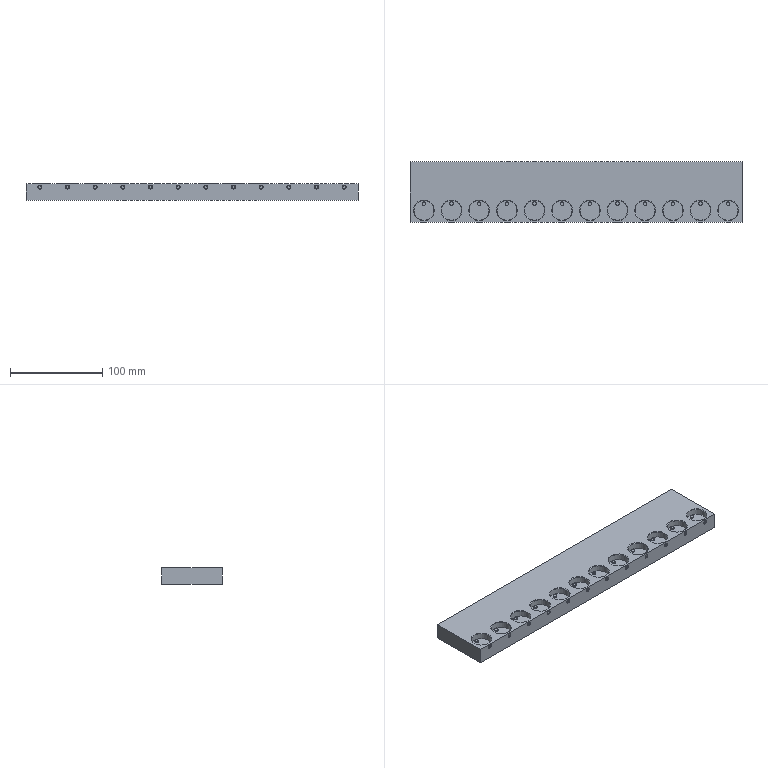NC program | NX | posted with a generic post | part box 360 x 66 x 17.6 mm
Lines 4604 to 5333 of 61781:
(2 , TOOL : D1-T2)
N9140 T02 M6
N9142 G54
N9144 G17 G0 G90 X-15.846 Y-13.281 B0. C0. S8000 M3
N9146 G43 Z100. H2
N9148 G94 G1 Z-5.5 F5000.
N9150 G3 X-15.846 Y-13.281 Z-5.515 I0.443 J0.081 F2000.
N9152 X-15.846 Y-13.281 Z-5.53 I0.443 J0.081
N9154 X-15.846 Y-13.281 Z-5.544 I0.443 J0.081
N9156 X-15.846 Y-13.281 Z-5.559 I0.443 J0.081
N9158 X-15.846 Y-13.281 Z-5.574 I0.443 J0.081
N9160 X-15.846 Y-13.281 Z-5.589 I0.443 J0.081
N9162 X-15.846 Y-13.281 Z-5.604 I0.443 J0.081
N9164 X-15.846 Y-13.281 Z-5.618 I0.443 J0.081
N9166 X-15.846 Y-13.281 Z-5.633 I0.443 J0.081
N9168 X-15.846 Y-13.281 Z-5.648 I0.443 J0.081
N9170 X-15.846 Y-13.281 Z-5.663 I0.443 J0.081
N9172 X-15.846 Y-13.281 Z-5.678 I0.443 J0.081
N9174 X-15. Y-13. Z-5.686 R-0.45
N9176 G1 X-14.874 Y-13.432
N9178 G3 X-14.568 Y-12.874 R0.45
N9180 X-14.874 Y-13.432 R-0.45
N9182 G1 X-14.706 Y-14.008
N9184 G3 X-13.992 Y-12.706 R1.05
N9186 X-14.706 Y-14.008 R-1.05
N9188 G1 X-14.537 Y-14.584
N9190 G3 X-13.416 Y-12.537 R1.65
N9192 X-14.537 Y-14.584 R-1.65
N9194 G1 X-14.369 Y-15.16
N9196 G3 X-12.84 Y-12.369 R2.25
N9198 X-14.369 Y-15.16 R-2.25
N9200 G1 X-14.201 Y-15.736
N9202 G3 X-12.264 Y-12.201 R2.85
N9204 X-14.201 Y-15.736 R-2.85
N9206 G1 X-14.032 Y-16.312
N9208 G3 X-11.688 Y-12.032 R3.45
N9210 X-14.032 Y-16.312 R-3.45
N9212 G1 X-13.864 Y-16.887
N9214 G3 X-11.113 Y-11.864 R4.05
N9216 X-13.864 Y-16.887 R-4.05
N9218 G1 X-13.696 Y-17.463
N9220 G3 X-10.537 Y-11.696 R4.65
N9222 X-13.696 Y-17.463 R-4.65
N9224 G1 X-13.528 Y-18.039
N9226 G3 X-9.961 Y-11.528 R5.25
N9228 X-13.528 Y-18.039 R-5.25
N9230 G1 X-13.359 Y-18.615
N9232 G3 X-9.385 Y-11.359 R5.85
N9234 X-13.359 Y-18.615 R-5.85
N9236 G1 X-13.191 Y-19.191
N9238 G3 X-8.809 Y-11.191 R6.45
N9240 X-13.191 Y-19.191 R-6.45
N9242 G1 X-13.023 Y-19.767
N9244 G3 X-8.233 Y-11.023 R7.05
N9246 X-13.023 Y-19.767 R-7.05
N9248 G1 X-12.854 Y-20.343
N9250 G3 X-7.657 Y-10.854 R7.65
N9252 X-12.854 Y-20.343 R-7.65
N9254 G1 X-12.686 Y-20.919
N9256 G3 X-7.081 Y-10.686 R8.25
N9258 X-12.686 Y-20.919 R-8.25
N9260 G1 X-12.518 Y-21.495
N9262 G3 X-6.505 Y-10.518 R8.85
N9264 X-12.518 Y-21.495 R-8.85
N9266 G1 X-12.35 Y-22.071
N9268 G3 X-5.929 Y-10.35 R9.45
N9270 X-12.35 Y-22.071 R-9.45
N9272 G1 X-12.181 Y-22.647
N9274 G3 X-5.353 Y-10.181 R10.05
N9276 X-12.181 Y-22.647 R-10.05
N9278 G1 X-12.321 Y-22.167
N9280 G0 Z100.
N9282 X-15.124 Y-11.483
N9284 G1 Z-5.686 F5000.
N9286 G3 X-15.124 Y-11.483 Z-5.701 I0.124 J0.433 F2000.
N9288 X-15.124 Y-11.483 Z-5.715 I0.124 J0.433
N9290 X-15.124 Y-11.483 Z-5.73 I0.124 J0.433
N9292 X-15.124 Y-11.483 Z-5.745 I0.124 J0.433
N9294 X-15.124 Y-11.483 Z-5.76 I0.124 J0.433
N9296 X-15.124 Y-11.483 Z-5.775 I0.124 J0.433
N9298 X-15.124 Y-11.483 Z-5.789 I0.124 J0.433
N9300 X-15.124 Y-11.483 Z-5.804 I0.124 J0.433
N9302 X-15.124 Y-11.483 Z-5.819 I0.124 J0.433
N9304 X-15.124 Y-11.483 Z-5.834 I0.124 J0.433
N9306 X-15.124 Y-11.483 Z-5.849 I0.124 J0.433
N9308 X-15.124 Y-11.483 Z-5.863 I0.124 J0.433
N9310 X-15. Y-10.6 Z-5.871 R-0.45
N9312 X-15.663 Y-10.693 R2.4
N9314 G2 X-14.337 Y-10.693 R9.679
N9316 G3 X-15. Y-10.6 R2.4
N9318 G1 Y-10.15
N9320 G3 X-17.381 Y-11.433 R2.85
N9322 G2 X-12.619 Y-11.433 R9.229
N9324 G3 X-15. Y-10.15 R2.85
N9326 G1 Y-9.55
N9328 G3 X-18.401 Y-12.419 R3.45
N9330 G2 X-11.599 Y-12.419 R8.629
N9332 G3 X-15. Y-9.55 R3.45
N9334 G1 Y-8.95
N9336 G3 X-19.03 Y-13.405 R4.05
N9338 G2 X-10.97 Y-13.405 R8.029
N9340 G3 X-15. Y-8.95 R4.05
N9342 G1 Y-8.35
N9344 G3 X-19.437 Y-14.391 R4.65
N9346 G2 X-10.563 Y-14.391 R7.429
N9348 G3 X-15. Y-8.35 R4.65
N9350 G1 Y-7.75
N9352 G3 X-19.681 Y-15.377 R5.25
N9354 G2 X-10.319 Y-15.377 R6.829
N9356 G3 X-15. Y-7.75 R5.25
N9358 G1 Y-7.15
N9360 G3 X-19.786 Y-16.363 R5.85
N9362 G2 X-10.214 Y-16.363 R6.229
N9364 G3 X-15. Y-7.15 R5.85
N9366 G1 Y-6.55
N9368 G3 X-19.763 Y-17.349 R6.45
N9370 G2 X-10.237 Y-17.349 R5.629
N9372 G3 X-15. Y-6.55 R6.45
N9374 G1 Y-5.95
N9376 G3 X-19.608 Y-18.335 R7.05
N9378 G2 X-10.392 Y-18.335 R5.029
N9380 G3 X-15. Y-5.95 R7.05
N9382 G1 Y-5.35
N9384 G3 X-19.308 Y-19.322 R7.65
N9386 G2 X-10.692 Y-19.322 R4.429
N9388 G3 X-15. Y-5.35 R7.65
N9390 G1 Y-4.75
N9392 G3 X-18.829 Y-20.308 R8.25
N9394 G2 X-11.171 Y-20.308 R3.829
N9396 G3 X-15. Y-4.75 R8.25
N9398 G1 Y-4.15
N9400 G3 X-18.088 Y-21.294 R8.85
N9402 G2 X-11.912 Y-21.294 R-3.229
N9404 G3 X-15. Y-4.15 R8.85
N9406 G1 Y-3.55
N9408 G3 X-16.786 Y-22.28 R9.45
N9410 G2 X-13.214 Y-22.28 R-2.629
N9412 G1 X-13.296 Y-22.192
N9414 G2 X-16.842 Y-22.054 R2.509
N9416 X-13.296 Y-22.192 R-2.509
N9418 G1 X-13.214 Y-22.28
N9420 G3 X-15. Y-3.55 R9.45
N9422 G1 Y-2.95
N9424 G3 X-25.05 Y-13. R10.05
N9426 X-15. Y-2.95 R-10.05
N9428 G1 Y-3.45
N9430 G0 Z-2.686
N9432 X-13.997 Y-11.303
N9434 G1 Z-5.871 F5000.
N9436 G3 X-13.997 Y-11.303 Z-5.886 I0.346 J0.288 F2000.
N9438 X-13.997 Y-11.303 Z-5.901 I0.346 J0.288
N9440 X-13.997 Y-11.303 Z-5.916 I0.346 J0.288
N9442 X-13.997 Y-11.303 Z-5.931 I0.346 J0.288
N9444 X-13.997 Y-11.303 Z-5.945 I0.346 J0.288
N9446 X-13.997 Y-11.303 Z-5.96 I0.346 J0.288
N9448 X-13.997 Y-11.303 Z-5.975 I0.346 J0.288
N9450 X-13.997 Y-11.303 Z-5.99 I0.346 J0.288
N9452 X-13.997 Y-11.303 Z-6.005 I0.346 J0.288
N9454 X-13.997 Y-11.303 Z-6.019 I0.346 J0.288
N9456 X-13.997 Y-11.303 Z-6.034 I0.346 J0.288
N9458 X-13.997 Y-11.303 Z-6.049 I0.346 J0.288
N9460 X-13.398 Y-10.643 Z-6.057 R-0.45
N9462 X-17.253 Y-11.255 R2.85
N9464 G2 X-12.747 Y-11.255 R9.37
N9466 G3 X-13.398 Y-10.643 R2.85
N9468 G1 X-13.061 Y-10.146
N9470 G3 X-18.368 Y-12.252 R3.45
N9472 G2 X-11.632 Y-12.252 R8.77
N9474 G3 X-13.061 Y-10.146 R3.45
N9476 G1 X-12.724 Y-9.65
N9478 G3 X-19.042 Y-13.25 R4.05
N9480 G2 X-10.958 Y-13.25 R8.17
N9482 G3 X-12.724 Y-9.65 R4.05
N9484 G1 X-12.387 Y-9.154
N9486 G3 X-19.48 Y-14.247 R4.65
N9488 G2 X-10.52 Y-14.247 R7.57
N9490 G3 X-12.387 Y-9.154 R4.65
N9492 G1 X-12.05 Y-8.657
N9494 G3 X-19.746 Y-15.245 R5.25
N9496 G2 X-10.254 Y-15.245 R6.97
N9498 G3 X-12.05 Y-8.657 R5.25
N9500 G1 X-11.712 Y-8.161
N9502 G3 X-19.869 Y-16.242 R5.85
N9504 G2 X-10.131 Y-16.242 R6.37
N9506 G3 X-11.712 Y-8.161 R5.85
N9508 G1 X-11.375 Y-7.665
N9510 G3 X-19.861 Y-17.24 R6.45
N9512 G2 X-10.139 Y-17.24 R5.77
N9514 G3 X-11.375 Y-7.665 R6.45
N9516 G1 X-11.038 Y-7.169
N9518 G3 X-19.719 Y-18.238 R7.05
N9520 G2 X-10.281 Y-18.238 R5.17
N9522 G3 X-11.038 Y-7.169 R7.05
N9524 G1 X-10.701 Y-6.672
N9526 G3 X-19.432 Y-19.235 R7.65
N9528 G2 X-10.568 Y-19.235 R4.57
N9530 G3 X-10.701 Y-6.672 R7.65
N9532 G1 X-10.364 Y-6.176
N9534 G3 X-18.969 Y-20.233 R-8.25
N9536 G2 X-11.031 Y-20.233 R3.97
N9538 G3 X-10.364 Y-6.176 R8.25
N9540 G1 X-10.026 Y-5.68
N9542 G3 X-18.253 Y-21.23 R-8.85
N9544 G2 X-11.747 Y-21.23 R-3.37
N9546 G3 X-10.026 Y-5.68 R8.85
N9548 G1 X-9.689 Y-5.183
N9550 G3 X-17.037 Y-22.228 R-9.45
N9552 G2 X-12.963 Y-22.228 R-2.77
N9554 G1 X-13.051 Y-22.147
N9556 G2 X-16.797 Y-22.299 R2.65
N9558 X-13.051 Y-22.147 R-2.65
N9560 G1 X-12.963 Y-22.228
N9562 G3 X-9.689 Y-5.183 R9.45
N9564 G1 X-9.352 Y-4.687
N9566 G3 X-23.313 Y-7.352 R10.05
N9568 X-9.352 Y-4.687 R-10.05
N9570 G1 X-9.633 Y-5.101
N9572 G0 Z-2.871
N9574 X-14.001 Y-11.301
N9576 G1 Z-6.057 F5000.
N9578 G3 X-14.001 Y-11.301 Z-6.072 I0.345 J0.289 F2000.
N9580 X-14.001 Y-11.301 Z-6.087 I0.345 J0.289
N9582 X-14.001 Y-11.301 Z-6.102 I0.345 J0.289
N9584 X-14.001 Y-11.301 Z-6.116 I0.345 J0.289
N9586 X-14.001 Y-11.301 Z-6.131 I0.345 J0.289
N9588 X-14.001 Y-11.301 Z-6.146 I0.345 J0.289
N9590 X-14.001 Y-11.301 Z-6.161 I0.345 J0.289
N9592 X-14.001 Y-11.301 Z-6.176 I0.345 J0.289
N9594 X-14.001 Y-11.301 Z-6.19 I0.345 J0.289
N9596 X-14.001 Y-11.301 Z-6.205 I0.345 J0.289
N9598 X-14.001 Y-11.301 Z-6.22 I0.345 J0.289
N9600 X-14.001 Y-11.301 Z-6.235 I0.345 J0.289
N9602 X-13.403 Y-10.639 Z-6.243 R-0.45
N9604 X-17.248 Y-11.249 R2.85
N9606 G2 X-12.752 Y-11.249 R9.375
N9608 G3 X-13.403 Y-10.639 R2.85
N9610 G1 X-13.067 Y-10.142
N9612 G3 X-18.367 Y-12.247 R3.45
N9614 G2 X-11.633 Y-12.247 R8.775
N9616 G3 X-13.067 Y-10.142 R3.45
N9618 G1 X-12.731 Y-9.645
N9620 G3 X-19.043 Y-13.245 R4.05
N9622 G2 X-10.957 Y-13.245 R8.175
N9624 G3 X-12.731 Y-9.645 R4.05
N9626 G1 X-12.395 Y-9.148
N9628 G3 X-19.481 Y-14.242 R4.65
N9630 G2 X-10.519 Y-14.242 R7.575
N9632 G3 X-12.395 Y-9.148 R4.65
N9634 G1 X-12.059 Y-8.651
N9636 G3 X-19.748 Y-15.24 R5.25
N9638 G2 X-10.252 Y-15.24 R6.975
N9640 G3 X-12.059 Y-8.651 R5.25
N9642 G1 X-11.723 Y-8.154
N9644 G3 X-19.872 Y-16.238 R5.85
N9646 G2 X-10.128 Y-16.238 R6.375
N9648 G3 X-11.723 Y-8.154 R5.85
N9650 G1 X-11.387 Y-7.657
N9652 G3 X-19.864 Y-17.236 R6.45
N9654 G2 X-10.136 Y-17.236 R5.775
N9656 G3 X-11.387 Y-7.657 R6.45
N9658 G1 X-11.051 Y-7.16
N9660 G3 X-19.723 Y-18.234 R7.05
N9662 G2 X-10.277 Y-18.234 R5.175
N9664 G3 X-11.051 Y-7.16 R7.05
N9666 G1 X-10.715 Y-6.663
N9668 G3 X-19.436 Y-19.232 R7.65
N9670 G2 X-10.564 Y-19.232 R4.575
N9672 G3 X-10.715 Y-6.663 R7.65
N9674 G1 X-10.378 Y-6.166
N9676 G3 X-18.973 Y-20.23 R-8.25
N9678 G2 X-11.027 Y-20.23 R3.975
N9680 G3 X-10.378 Y-6.166 R8.25
N9682 G1 X-10.042 Y-5.669
N9684 G3 X-18.259 Y-21.228 R-8.85
N9686 G2 X-11.741 Y-21.228 R-3.375
N9688 G3 X-10.042 Y-5.669 R8.85
N9690 G1 X-9.706 Y-5.172
N9692 G3 X-17.045 Y-22.226 R-9.45
N9694 G2 X-12.955 Y-22.226 R-2.775
N9696 G1 X-13.044 Y-22.145
N9698 G2 X-16.795 Y-22.306 R2.655
N9700 X-13.044 Y-22.145 R-2.655
N9702 G1 X-12.955 Y-22.226
N9704 G3 X-9.706 Y-5.172 R9.45
N9706 G1 X-9.37 Y-4.675
N9708 G3 X-23.325 Y-7.37 R10.05
N9710 X-9.37 Y-4.675 R-10.05
N9712 G1 X-9.65 Y-5.089
N9714 G0 Z-3.057
N9716 X-14.001 Y-11.301
N9718 G1 Z-6.243 F5000.
N9720 G3 X-14.001 Y-11.301 Z-6.258 I0.345 J0.289 F2000.
N9722 X-14.001 Y-11.301 Z-6.272 I0.345 J0.289
N9724 X-14.001 Y-11.301 Z-6.287 I0.345 J0.289
N9726 X-14.001 Y-11.301 Z-6.302 I0.345 J0.289
N9728 X-14.001 Y-11.301 Z-6.317 I0.345 J0.289
N9730 X-14.001 Y-11.301 Z-6.332 I0.345 J0.289
N9732 X-14.001 Y-11.301 Z-6.346 I0.345 J0.289
N9734 X-14.001 Y-11.301 Z-6.361 I0.345 J0.289
N9736 X-14.001 Y-11.301 Z-6.376 I0.345 J0.289
N9738 X-14.001 Y-11.301 Z-6.391 I0.345 J0.289
N9740 X-14.001 Y-11.301 Z-6.406 I0.345 J0.289
N9742 X-14.001 Y-11.301 Z-6.421 I0.345 J0.289
N9744 X-13.403 Y-10.639 Z-6.429 R-0.45
N9746 X-17.248 Y-11.249 R2.85
N9748 G2 X-12.752 Y-11.249 R9.375
N9750 G3 X-13.403 Y-10.639 R2.85
N9752 G1 X-13.067 Y-10.142
N9754 G3 X-18.367 Y-12.247 R3.45
N9756 G2 X-11.633 Y-12.247 R8.775
N9758 G3 X-13.067 Y-10.142 R3.45
N9760 G1 X-12.731 Y-9.645
N9762 G3 X-19.043 Y-13.245 R4.05
N9764 G2 X-10.957 Y-13.245 R8.175
N9766 G3 X-12.731 Y-9.645 R4.05
N9768 G1 X-12.395 Y-9.148
N9770 G3 X-19.481 Y-14.242 R4.65
N9772 G2 X-10.519 Y-14.242 R7.575
N9774 G3 X-12.395 Y-9.148 R4.65
N9776 G1 X-12.059 Y-8.651
N9778 G3 X-19.748 Y-15.24 R5.25
N9780 G2 X-10.252 Y-15.24 R6.975
N9782 G3 X-12.059 Y-8.651 R5.25
N9784 G1 X-11.723 Y-8.154
N9786 G3 X-19.872 Y-16.238 R5.85
N9788 G2 X-10.128 Y-16.238 R6.375
N9790 G3 X-11.723 Y-8.154 R5.85
N9792 G1 X-11.387 Y-7.657
N9794 G3 X-19.864 Y-17.236 R6.45
N9796 G2 X-10.136 Y-17.236 R5.775
N9798 G3 X-11.387 Y-7.657 R6.45
N9800 G1 X-11.051 Y-7.16
N9802 G3 X-19.723 Y-18.234 R7.05
N9804 G2 X-10.277 Y-18.234 R5.175
N9806 G3 X-11.051 Y-7.16 R7.05
N9808 G1 X-10.715 Y-6.663
N9810 G3 X-19.436 Y-19.232 R7.65
N9812 G2 X-10.564 Y-19.232 R4.575
N9814 G3 X-10.715 Y-6.663 R7.65
N9816 G1 X-10.378 Y-6.166
N9818 G3 X-18.973 Y-20.23 R-8.25
N9820 G2 X-11.027 Y-20.23 R3.975
N9822 G3 X-10.378 Y-6.166 R8.25
N9824 G1 X-10.042 Y-5.669
N9826 G3 X-18.259 Y-21.228 R-8.85
N9828 G2 X-11.741 Y-21.228 R-3.375
N9830 G3 X-10.042 Y-5.669 R8.85
N9832 G1 X-9.706 Y-5.172
N9834 G3 X-17.045 Y-22.226 R-9.45
N9836 G2 X-12.955 Y-22.226 R-2.775
N9838 G1 X-13.044 Y-22.145
N9840 G2 X-16.795 Y-22.306 R2.655
N9842 X-13.044 Y-22.145 R-2.655
N9844 G1 X-12.955 Y-22.226
N9846 G3 X-9.706 Y-5.172 R9.45
N9848 G1 X-9.37 Y-4.675
N9850 G3 X-23.325 Y-7.37 R10.05
N9852 X-9.37 Y-4.675 R-10.05
N9854 G1 X-9.65 Y-5.089
N9856 G0 Z-3.243
N9858 X-14.001 Y-11.301
N9860 G1 Z-6.429 F5000.
N9862 G3 X-14.001 Y-11.301 Z-6.443 I0.345 J0.289 F2000.
N9864 X-14.001 Y-11.301 Z-6.458 I0.345 J0.289
N9866 X-14.001 Y-11.301 Z-6.473 I0.345 J0.289
N9868 X-14.001 Y-11.301 Z-6.488 I0.345 J0.289
N9870 X-14.001 Y-11.301 Z-6.503 I0.345 J0.289
N9872 X-14.001 Y-11.301 Z-6.517 I0.345 J0.289
N9874 X-14.001 Y-11.301 Z-6.532 I0.345 J0.289
N9876 X-14.001 Y-11.301 Z-6.547 I0.345 J0.289
N9878 X-14.001 Y-11.301 Z-6.562 I0.345 J0.289
N9880 X-14.001 Y-11.301 Z-6.577 I0.345 J0.289
N9882 X-14.001 Y-11.301 Z-6.591 I0.345 J0.289
N9884 X-14.001 Y-11.301 Z-6.606 I0.345 J0.289
N9886 X-13.403 Y-10.639 Z-6.614 R-0.45
N9888 X-17.248 Y-11.249 R2.85
N9890 G2 X-12.752 Y-11.249 R9.375
N9892 G3 X-13.403 Y-10.639 R2.85
N9894 G1 X-13.067 Y-10.142
N9896 G3 X-18.367 Y-12.247 R3.45
N9898 G2 X-11.633 Y-12.247 R8.775
N9900 G3 X-13.067 Y-10.142 R3.45
N9902 G1 X-12.731 Y-9.645
N9904 G3 X-19.043 Y-13.245 R4.05
N9906 G2 X-10.957 Y-13.245 R8.175
N9908 G3 X-12.731 Y-9.645 R4.05
N9910 G1 X-12.395 Y-9.148
N9912 G3 X-19.481 Y-14.242 R4.65
N9914 G2 X-10.519 Y-14.242 R7.575
N9916 G3 X-12.395 Y-9.148 R4.65
N9918 G1 X-12.059 Y-8.651
N9920 G3 X-19.748 Y-15.24 R5.25
N9922 G2 X-10.252 Y-15.24 R6.975
N9924 G3 X-12.059 Y-8.651 R5.25
N9926 G1 X-11.723 Y-8.154
N9928 G3 X-19.872 Y-16.238 R5.85
N9930 G2 X-10.128 Y-16.238 R6.375
N9932 G3 X-11.723 Y-8.154 R5.85
N9934 G1 X-11.387 Y-7.657
N9936 G3 X-19.864 Y-17.236 R6.45
N9938 G2 X-10.136 Y-17.236 R5.775
N9940 G3 X-11.387 Y-7.657 R6.45
N9942 G1 X-11.051 Y-7.16
N9944 G3 X-19.723 Y-18.234 R7.05
N9946 G2 X-10.277 Y-18.234 R5.175
N9948 G3 X-11.051 Y-7.16 R7.05
N9950 G1 X-10.715 Y-6.663
N9952 G3 X-19.436 Y-19.232 R7.65
N9954 G2 X-10.564 Y-19.232 R4.575
N9956 G3 X-10.715 Y-6.663 R7.65
N9958 G1 X-10.378 Y-6.166
N9960 G3 X-18.973 Y-20.23 R-8.25
N9962 G2 X-11.027 Y-20.23 R3.975
N9964 G3 X-10.378 Y-6.166 R8.25
N9966 G1 X-10.042 Y-5.669
N9968 G3 X-18.259 Y-21.228 R-8.85
N9970 G2 X-11.741 Y-21.228 R-3.375
N9972 G3 X-10.042 Y-5.669 R8.85
N9974 G1 X-9.706 Y-5.172
N9976 G3 X-17.045 Y-22.226 R-9.45
N9978 G2 X-12.955 Y-22.226 R-2.775
N9980 G1 X-13.044 Y-22.145
N9982 G2 X-16.795 Y-22.306 R2.655
N9984 X-13.044 Y-22.145 R-2.655
N9986 G1 X-12.955 Y-22.226
N9988 G3 X-9.706 Y-5.172 R9.45
N9990 G1 X-9.37 Y-4.675
N9992 G3 X-23.325 Y-7.37 R10.05
N9994 X-9.37 Y-4.675 R-10.05
N9996 G1 X-9.65 Y-5.089
N9998 G0 Z-3.429
N10000 X-14.001 Y-11.301
N10002 G1 Z-6.614 F5000.
N10004 G3 X-14.001 Y-11.301 Z-6.629 I0.345 J0.289 F2000.
N10006 X-14.001 Y-11.301 Z-6.644 I0.345 J0.289
N10008 X-14.001 Y-11.301 Z-6.659 I0.345 J0.289
N10010 X-14.001 Y-11.301 Z-6.674 I0.345 J0.289
N10012 X-14.001 Y-11.301 Z-6.688 I0.345 J0.289
N10014 X-14.001 Y-11.301 Z-6.703 I0.345 J0.289
N10016 X-14.001 Y-11.301 Z-6.718 I0.345 J0.289
N10018 X-14.001 Y-11.301 Z-6.733 I0.345 J0.289
N10020 X-14.001 Y-11.301 Z-6.748 I0.345 J0.289
N10022 X-14.001 Y-11.301 Z-6.762 I0.345 J0.289
N10024 X-14.001 Y-11.301 Z-6.777 I0.345 J0.289
N10026 X-14.001 Y-11.301 Z-6.792 I0.345 J0.289
N10028 X-13.403 Y-10.639 Z-6.8 R-0.45
N10030 X-17.248 Y-11.249 R2.85
N10032 G2 X-12.752 Y-11.249 R9.375
N10034 G3 X-13.403 Y-10.639 R2.85
N10036 G1 X-13.067 Y-10.142
N10038 G3 X-18.367 Y-12.247 R3.45
N10040 G2 X-11.633 Y-12.247 R8.775
N10042 G3 X-13.067 Y-10.142 R3.45
N10044 G1 X-12.731 Y-9.645
N10046 G3 X-19.043 Y-13.245 R4.05
N10048 G2 X-10.957 Y-13.245 R8.175
N10050 G3 X-12.731 Y-9.645 R4.05
N10052 G1 X-12.395 Y-9.148
N10054 G3 X-19.481 Y-14.242 R4.65
N10056 G2 X-10.519 Y-14.242 R7.575
N10058 G3 X-12.395 Y-9.148 R4.65
N10060 G1 X-12.059 Y-8.651
N10062 G3 X-19.748 Y-15.24 R5.25
N10064 G2 X-10.252 Y-15.24 R6.975
N10066 G3 X-12.059 Y-8.651 R5.25
N10068 G1 X-11.723 Y-8.154
N10070 G3 X-19.872 Y-16.238 R5.85
N10072 G2 X-10.128 Y-16.238 R6.375
N10074 G3 X-11.723 Y-8.154 R5.85
N10076 G1 X-11.387 Y-7.657
N10078 G3 X-19.864 Y-17.236 R6.45
N10080 G2 X-10.136 Y-17.236 R5.775
N10082 G3 X-11.387 Y-7.657 R6.45
N10084 G1 X-11.051 Y-7.16
N10086 G3 X-19.723 Y-18.234 R7.05
N10088 G2 X-10.277 Y-18.234 R5.175
N10090 G3 X-11.051 Y-7.16 R7.05
N10092 G1 X-10.715 Y-6.663
N10094 G3 X-19.436 Y-19.232 R7.65
N10096 G2 X-10.564 Y-19.232 R4.575
N10098 G3 X-10.715 Y-6.663 R7.65
N10100 G1 X-10.378 Y-6.166
N10102 G3 X-18.973 Y-20.23 R-8.25
N10104 G2 X-11.027 Y-20.23 R3.975
N10106 G3 X-10.378 Y-6.166 R8.25
N10108 G1 X-10.042 Y-5.669
N10110 G3 X-18.259 Y-21.228 R-8.85
N10112 G2 X-11.741 Y-21.228 R-3.375
N10114 G3 X-10.042 Y-5.669 R8.85
N10116 G1 X-9.706 Y-5.172
N10118 G3 X-17.045 Y-22.226 R-9.45
N10120 G2 X-12.955 Y-22.226 R-2.775
N10122 G1 X-13.044 Y-22.145
N10124 G2 X-16.795 Y-22.306 R2.655
N10126 X-13.044 Y-22.145 R-2.655
N10128 G1 X-12.955 Y-22.226
N10130 G3 X-9.706 Y-5.172 R9.45
N10132 G1 X-9.37 Y-4.675
N10134 G3 X-23.325 Y-7.37 R10.05
N10136 X-9.37 Y-4.675 R-10.05
N10138 G1 X-9.65 Y-5.089
N10140 G0 Z100.
(2_COPY , TOOL : D1-T2)
N10142 X-45.846 Y-13.281
N10144 G1 Z-5.5 F5000.
N10146 G3 X-45.846 Y-13.281 Z-5.515 I0.443 J0.081 F2000.
N10148 X-45.846 Y-13.281 Z-5.53 I0.443 J0.081
N10150 X-45.846 Y-13.281 Z-5.544 I0.443 J0.081
N10152 X-45.846 Y-13.281 Z-5.559 I0.443 J0.081
N10154 X-45.846 Y-13.281 Z-5.574 I0.443 J0.081
N10156 X-45.846 Y-13.281 Z-5.589 I0.443 J0.081
N10158 X-45.846 Y-13.281 Z-5.604 I0.443 J0.081
N10160 X-45.846 Y-13.281 Z-5.618 I0.443 J0.081
N10162 X-45.846 Y-13.281 Z-5.633 I0.443 J0.081
N10164 X-45.846 Y-13.281 Z-5.648 I0.443 J0.081
N10166 X-45.846 Y-13.281 Z-5.663 I0.443 J0.081
N10168 X-45.846 Y-13.281 Z-5.678 I0.443 J0.081
N10170 X-45. Y-13. Z-5.686 R-0.45
N10172 G1 X-44.874 Y-13.432
N10174 G3 X-44.568 Y-12.874 R0.45
N10176 X-44.874 Y-13.432 R-0.45
N10178 G1 X-44.706 Y-14.008
N10180 G3 X-43.992 Y-12.706 R1.05
N10182 X-44.706 Y-14.008 R-1.05
N10184 G1 X-44.537 Y-14.584
N10186 G3 X-43.416 Y-12.537 R1.65
N10188 X-44.537 Y-14.584 R-1.65
N10190 G1 X-44.369 Y-15.16
N10192 G3 X-42.84 Y-12.369 R2.25
N10194 X-44.369 Y-15.16 R-2.25
N10196 G1 X-44.201 Y-15.736
N10198 G3 X-42.264 Y-12.201 R2.85
N10200 X-44.201 Y-15.736 R-2.85
N10202 G1 X-44.032 Y-16.312
N10204 G3 X-41.688 Y-12.032 R3.45
N10206 X-44.032 Y-16.312 R-3.45
N10208 G1 X-43.864 Y-16.887
N10210 G3 X-41.113 Y-11.864 R4.05
N10212 X-43.864 Y-16.887 R-4.05
N10214 G1 X-43.696 Y-17.463
N10216 G3 X-40.537 Y-11.696 R4.65
N10218 X-43.696 Y-17.463 R-4.65
N10220 G1 X-43.528 Y-18.039
N10222 G3 X-39.961 Y-11.528 R5.25
N10224 X-43.528 Y-18.039 R-5.25
N10226 G1 X-43.359 Y-18.615
N10228 G3 X-39.385 Y-11.359 R5.85
N10230 X-43.359 Y-18.615 R-5.85
N10232 G1 X-43.191 Y-19.191
N10234 G3 X-38.809 Y-11.191 R6.45
N10236 X-43.191 Y-19.191 R-6.45
N10238 G1 X-43.023 Y-19.767
N10240 G3 X-38.233 Y-11.023 R7.05
N10242 X-43.023 Y-19.767 R-7.05
N10244 G1 X-42.854 Y-20.343
N10246 G3 X-37.657 Y-10.854 R7.65
N10248 X-42.854 Y-20.343 R-7.65
N10250 G1 X-42.686 Y-20.919
N10252 G3 X-37.081 Y-10.686 R8.25
N10254 X-42.686 Y-20.919 R-8.25
N10256 G1 X-42.518 Y-21.495
N10258 G3 X-36.505 Y-10.518 R8.85
N10260 X-42.518 Y-21.495 R-8.85
N10262 G1 X-42.35 Y-22.071
N10264 G3 X-35.929 Y-10.35 R9.45
N10266 X-42.35 Y-22.071 R-9.45
N10268 G1 X-42.181 Y-22.647
N10270 G3 X-35.353 Y-10.181 R10.05
N10272 X-42.181 Y-22.647 R-10.05
N10274 G1 X-42.321 Y-22.167
N10276 G0 Z100.
N10278 X-45.124 Y-11.483
N10280 G1 Z-5.686 F5000.
N10282 G3 X-45.124 Y-11.483 Z-5.701 I0.124 J0.433 F2000.
N10284 X-45.124 Y-11.483 Z-5.715 I0.124 J0.433
N10286 X-45.124 Y-11.483 Z-5.73 I0.124 J0.433
N10288 X-45.124 Y-11.483 Z-5.745 I0.124 J0.433
N10290 X-45.124 Y-11.483 Z-5.76 I0.124 J0.433
N10292 X-45.124 Y-11.483 Z-5.775 I0.124 J0.433
N10294 X-45.124 Y-11.483 Z-5.789 I0.124 J0.433
N10296 X-45.124 Y-11.483 Z-5.804 I0.124 J0.433
N10298 X-45.124 Y-11.483 Z-5.819 I0.124 J0.433
N10300 X-45.124 Y-11.483 Z-5.834 I0.124 J0.433
N10302 X-45.124 Y-11.483 Z-5.849 I0.124 J0.433
N10304 X-45.124 Y-11.483 Z-5.863 I0.124 J0.433
N10306 X-45. Y-10.6 Z-5.871 R-0.45
N10308 X-45.663 Y-10.693 R2.4
N10310 G2 X-44.337 Y-10.693 R9.679
N10312 G3 X-45. Y-10.6 R2.4
N10314 G1 Y-10.15
N10316 G3 X-47.381 Y-11.433 R2.85
N10318 G2 X-42.619 Y-11.433 R9.229
N10320 G3 X-45. Y-10.15 R2.85
N10322 G1 Y-9.55
N10324 G3 X-48.401 Y-12.419 R3.45
N10326 G2 X-41.599 Y-12.419 R8.629
N10328 G3 X-45. Y-9.55 R3.45
N10330 G1 Y-8.95
N10332 G3 X-49.03 Y-13.405 R4.05
N10334 G2 X-40.97 Y-13.405 R8.029
N10336 G3 X-45. Y-8.95 R4.05
N10338 G1 Y-8.35
N10340 G3 X-49.437 Y-14.391 R4.65
N10342 G2 X-40.563 Y-14.391 R7.429
N10344 G3 X-45. Y-8.35 R4.65
N10346 G1 Y-7.75
N10348 G3 X-49.681 Y-15.377 R5.25
N10350 G2 X-40.319 Y-15.377 R6.829
N10352 G3 X-45. Y-7.75 R5.25
N10354 G1 Y-7.15
N10356 G3 X-49.786 Y-16.363 R5.85
N10358 G2 X-40.214 Y-16.363 R6.229
N10360 G3 X-45. Y-7.15 R5.85
N10362 G1 Y-6.55
N10364 G3 X-49.763 Y-17.349 R6.45
N10366 G2 X-40.237 Y-17.349 R5.629
N10368 G3 X-45. Y-6.55 R6.45
N10370 G1 Y-5.95
N10372 G3 X-49.608 Y-18.335 R7.05
N10374 G2 X-40.392 Y-18.335 R5.029
N10376 G3 X-45. Y-5.95 R7.05
N10378 G1 Y-5.35
N10380 G3 X-49.308 Y-19.322 R7.65
N10382 G2 X-40.692 Y-19.322 R4.429
N10384 G3 X-45. Y-5.35 R7.65
N10386 G1 Y-4.75
N10388 G3 X-48.829 Y-20.308 R8.25
N10390 G2 X-41.171 Y-20.308 R3.829
N10392 G3 X-45. Y-4.75 R8.25
N10394 G1 Y-4.15
N10396 G3 X-48.088 Y-21.294 R8.85
N10398 G2 X-41.912 Y-21.294 R-3.229
N10400 G3 X-45. Y-4.15 R8.85
N10402 G1 Y-3.55
N10404 G3 X-46.786 Y-22.28 R9.45
N10406 G2 X-43.214 Y-22.28 R-2.629
N10408 G1 X-43.296 Y-22.192
N10410 G2 X-46.842 Y-22.054 R2.509
N10412 X-43.296 Y-22.192 R-2.509
N10414 G1 X-43.214 Y-22.28
N10416 G3 X-45. Y-3.55 R9.45
N10418 G1 Y-2.95
N10420 G3 X-55.05 Y-13. R10.05
N10422 X-45. Y-2.95 R-10.05
N10424 G1 Y-3.45
N10426 G0 Z-2.686
N10428 X-43.997 Y-11.303
N10430 G1 Z-5.871 F5000.
N10432 G3 X-43.997 Y-11.303 Z-5.886 I0.346 J0.288 F2000.
N10434 X-43.997 Y-11.303 Z-5.901 I0.346 J0.288
N10436 X-43.997 Y-11.303 Z-5.916 I0.346 J0.288
N10438 X-43.997 Y-11.303 Z-5.931 I0.346 J0.288
N10440 X-43.997 Y-11.303 Z-5.945 I0.346 J0.288
N10442 X-43.997 Y-11.303 Z-5.96 I0.346 J0.288
N10444 X-43.997 Y-11.303 Z-5.975 I0.346 J0.288
N10446 X-43.997 Y-11.303 Z-5.99 I0.346 J0.288
N10448 X-43.997 Y-11.303 Z-6.005 I0.346 J0.288
N10450 X-43.997 Y-11.303 Z-6.019 I0.346 J0.288
N10452 X-43.997 Y-11.303 Z-6.034 I0.346 J0.288
N10454 X-43.997 Y-11.303 Z-6.049 I0.346 J0.288
N10456 X-43.398 Y-10.643 Z-6.057 R-0.45
N10458 X-47.253 Y-11.255 R2.85
N10460 G2 X-42.747 Y-11.255 R9.37
N10462 G3 X-43.398 Y-10.643 R2.85
N10464 G1 X-43.061 Y-10.146
N10466 G3 X-48.368 Y-12.252 R3.45
N10468 G2 X-41.632 Y-12.252 R8.77
N10470 G3 X-43.061 Y-10.146 R3.45
N10472 G1 X-42.724 Y-9.65
N10474 G3 X-49.042 Y-13.25 R4.05
N10476 G2 X-40.958 Y-13.25 R8.17
N10478 G3 X-42.724 Y-9.65 R4.05
N10480 G1 X-42.387 Y-9.154
N10482 G3 X-49.48 Y-14.247 R4.65
N10484 G2 X-40.52 Y-14.247 R7.57
N10486 G3 X-42.387 Y-9.154 R4.65
N10488 G1 X-42.05 Y-8.657
N10490 G3 X-49.746 Y-15.245 R5.25
N10492 G2 X-40.254 Y-15.245 R6.97
N10494 G3 X-42.05 Y-8.657 R5.25
N10496 G1 X-41.712 Y-8.161
N10498 G3 X-49.869 Y-16.242 R5.85
N10500 G2 X-40.131 Y-16.242 R6.37
N10502 G3 X-41.712 Y-8.161 R5.85
N10504 G1 X-41.375 Y-7.665
N10506 G3 X-49.861 Y-17.24 R6.45
N10508 G2 X-40.139 Y-17.24 R5.77
N10510 G3 X-41.375 Y-7.665 R6.45
N10512 G1 X-41.038 Y-7.169
N10514 G3 X-49.719 Y-18.238 R7.05
N10516 G2 X-40.281 Y-18.238 R5.17
N10518 G3 X-41.038 Y-7.169 R7.05
N10520 G1 X-40.701 Y-6.672
N10522 G3 X-49.432 Y-19.235 R7.65
N10524 G2 X-40.568 Y-19.235 R4.57
N10526 G3 X-40.701 Y-6.672 R7.65
N10528 G1 X-40.364 Y-6.176
N10530 G3 X-48.969 Y-20.233 R-8.25
N10532 G2 X-41.031 Y-20.233 R3.97
N10534 G3 X-40.364 Y-6.176 R8.25
N10536 G1 X-40.026 Y-5.68
N10538 G3 X-48.253 Y-21.23 R-8.85
N10540 G2 X-41.747 Y-21.23 R-3.37
N10542 G3 X-40.026 Y-5.68 R8.85
N10544 G1 X-39.689 Y-5.183
N10546 G3 X-47.037 Y-22.228 R-9.45
N10548 G2 X-42.963 Y-22.228 R-2.77
N10550 G1 X-43.051 Y-22.147
N10552 G2 X-46.797 Y-22.299 R2.65
N10554 X-43.051 Y-22.147 R-2.65
N10556 G1 X-42.963 Y-22.228
N10558 G3 X-39.689 Y-5.183 R9.45
N10560 G1 X-39.352 Y-4.687
N10562 G3 X-53.313 Y-7.352 R10.05
N10564 X-39.352 Y-4.687 R-10.05
N10566 G1 X-39.633 Y-5.101
N10568 G0 Z-2.871
N10570 X-44.001 Y-11.301
N10572 G1 Z-6.057 F5000.
N10574 G3 X-44.001 Y-11.301 Z-6.072 I0.345 J0.289 F2000.
N10576 X-44.001 Y-11.301 Z-6.087 I0.345 J0.289
N10578 X-44.001 Y-11.301 Z-6.102 I0.345 J0.289
N10580 X-44.001 Y-11.301 Z-6.116 I0.345 J0.289
N10582 X-44.001 Y-11.301 Z-6.131 I0.345 J0.289
N10584 X-44.001 Y-11.301 Z-6.146 I0.345 J0.289
N10586 X-44.001 Y-11.301 Z-6.161 I0.345 J0.289